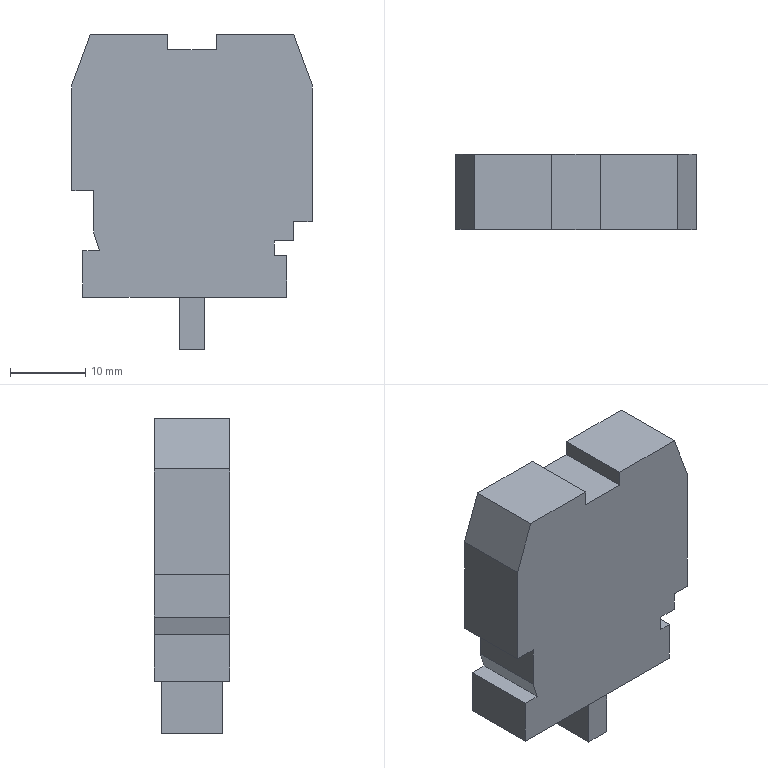Part | STEP file | 1 solid | 28 faces | box 32 x 10 x 42 mm | volume 10410 mm3 | plane 28